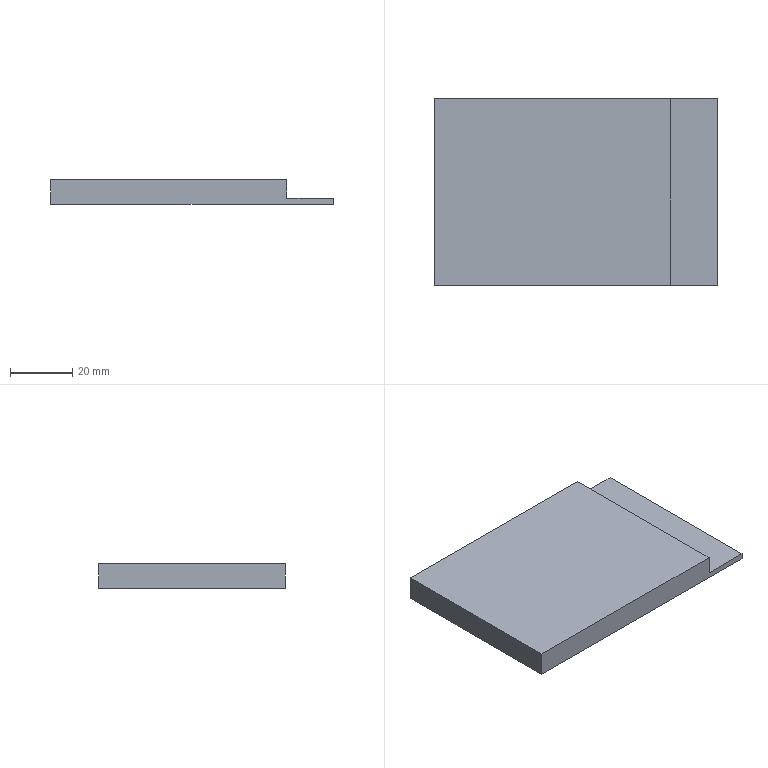Part | STEP file | Plate 4 | 1 solid | 8 faces | box 91 x 60 x 8 mm | volume 38280 mm3 | plane 8
STEP:
#1=CARTESIAN_POINT('',(45.5,30.,2.));
#2=VERTEX_POINT('',#1);
#3=CARTESIAN_POINT('',(45.5,30.,0.));
#4=VERTEX_POINT('',#3);
#5=CARTESIAN_POINT('',(45.5,30.,8.));
#6=DIRECTION('',(0.,0.,-1.));
#7=VECTOR('',#6,1000.);
#8=LINE('',#5,#7);
#9=EDGE_CURVE('',#2,#4,#8,.T.);
#10=ORIENTED_EDGE('',*,*,#9,.F.);
#11=CARTESIAN_POINT('',(45.5,-30.,2.));
#12=VERTEX_POINT('',#11);
#13=CARTESIAN_POINT('',(45.5,30.001,2.));
#14=DIRECTION('',(0.,-1.,0.));
#15=VECTOR('',#14,1000.);
#16=LINE('',#13,#15);
#17=EDGE_CURVE('',#2,#12,#16,.T.);
#18=ORIENTED_EDGE('',*,*,#17,.T.);
#19=CARTESIAN_POINT('',(45.5,-30.,0.));
#20=VERTEX_POINT('',#19);
#21=CARTESIAN_POINT('',(45.5,-30.,8.));
#22=DIRECTION('',(0.,0.,-1.));
#23=VECTOR('',#22,1000.);
#24=LINE('',#21,#23);
#25=EDGE_CURVE('',#12,#20,#24,.T.);
#26=ORIENTED_EDGE('',*,*,#25,.T.);
#27=CARTESIAN_POINT('',(45.5,-30.,0.));
#28=DIRECTION('',(0.,1.,0.));
#29=VECTOR('',#28,1000.);
#30=LINE('',#27,#29);
#31=EDGE_CURVE('',#20,#4,#30,.T.);
#32=ORIENTED_EDGE('',*,*,#31,.T.);
#33=EDGE_LOOP('',(#10,#18,#26,#32));
#34=FACE_OUTER_BOUND('',#33,.T.);
#35=CARTESIAN_POINT('',(45.5,-30.,8.));
#36=DIRECTION('',(-1.,0.,0.));
#37=DIRECTION('',(0.,0.,1.));
#38=AXIS2_PLACEMENT_3D('',#35,#36,#37);
#39=PLANE('',#38);
#40=ADVANCED_FACE('',(#34),#39,.F.);
#41=CARTESIAN_POINT('',(30.5,30.,2.));
#42=VERTEX_POINT('',#41);
#43=CARTESIAN_POINT('',(30.5,30.,8.));
#44=VERTEX_POINT('',#43);
#45=CARTESIAN_POINT('',(30.5,30.,8.));
#46=DIRECTION('',(0.,0.,1.));
#47=VECTOR('',#46,1000.);
#48=LINE('',#45,#47);
#49=EDGE_CURVE('',#42,#44,#48,.T.);
#50=ORIENTED_EDGE('',*,*,#49,.F.);
#51=CARTESIAN_POINT('',(45.5,30.,2.));
#52=DIRECTION('',(-1.,0.,0.));
#53=VECTOR('',#52,1000.);
#54=LINE('',#51,#53);
#55=EDGE_CURVE('',#2,#42,#54,.T.);
#56=ORIENTED_EDGE('',*,*,#55,.F.);
#57=ORIENTED_EDGE('',*,*,#9,.T.);
#58=CARTESIAN_POINT('',(-45.5,30.,0.));
#59=VERTEX_POINT('',#58);
#60=CARTESIAN_POINT('',(-45.5,30.,0.));
#61=DIRECTION('',(-1.,0.,0.));
#62=VECTOR('',#61,1000.);
#63=LINE('',#60,#62);
#64=EDGE_CURVE('',#4,#59,#63,.T.);
#65=ORIENTED_EDGE('',*,*,#64,.T.);
#66=CARTESIAN_POINT('',(-45.5,30.,8.));
#67=VERTEX_POINT('',#66);
#68=CARTESIAN_POINT('',(-45.5,30.,8.));
#69=DIRECTION('',(0.,0.,-1.));
#70=VECTOR('',#69,1000.);
#71=LINE('',#68,#70);
#72=EDGE_CURVE('',#67,#59,#71,.T.);
#73=ORIENTED_EDGE('',*,*,#72,.F.);
#74=CARTESIAN_POINT('',(-45.5,30.,8.));
#75=DIRECTION('',(-1.,0.,0.));
#76=VECTOR('',#75,1000.);
#77=LINE('',#74,#76);
#78=EDGE_CURVE('',#44,#67,#77,.T.);
#79=ORIENTED_EDGE('',*,*,#78,.F.);
#80=EDGE_LOOP('',(#50,#56,#57,#65,#73,#79));
#81=FACE_OUTER_BOUND('',#80,.T.);
#82=CARTESIAN_POINT('',(-45.5,30.,8.));
#83=DIRECTION('',(0.,-1.,0.));
#84=DIRECTION('',(0.,0.,-1.));
#85=AXIS2_PLACEMENT_3D('',#82,#83,#84);
#86=PLANE('',#85);
#87=ADVANCED_FACE('',(#81),#86,.F.);
#88=CARTESIAN_POINT('',(-45.5,-30.,0.));
#89=VERTEX_POINT('',#88);
#90=CARTESIAN_POINT('',(-45.5,-30.,0.));
#91=DIRECTION('',(0.,-1.,0.));
#92=VECTOR('',#91,1000.);
#93=LINE('',#90,#92);
#94=EDGE_CURVE('',#59,#89,#93,.T.);
#95=ORIENTED_EDGE('',*,*,#94,.T.);
#96=CARTESIAN_POINT('',(-45.5,-30.,8.));
#97=VERTEX_POINT('',#96);
#98=CARTESIAN_POINT('',(-45.5,-30.,8.));
#99=DIRECTION('',(0.,0.,-1.));
#100=VECTOR('',#99,1000.);
#101=LINE('',#98,#100);
#102=EDGE_CURVE('',#97,#89,#101,.T.);
#103=ORIENTED_EDGE('',*,*,#102,.F.);
#104=CARTESIAN_POINT('',(-45.5,-30.,8.));
#105=DIRECTION('',(0.,-1.,0.));
#106=VECTOR('',#105,1000.);
#107=LINE('',#104,#106);
#108=EDGE_CURVE('',#67,#97,#107,.T.);
#109=ORIENTED_EDGE('',*,*,#108,.F.);
#110=ORIENTED_EDGE('',*,*,#72,.T.);
#111=EDGE_LOOP('',(#95,#103,#109,#110));
#112=FACE_OUTER_BOUND('',#111,.T.);
#113=CARTESIAN_POINT('',(-45.5,-30.,8.));
#114=DIRECTION('',(1.,0.,0.));
#115=DIRECTION('',(0.,0.,-1.));
#116=AXIS2_PLACEMENT_3D('',#113,#114,#115);
#117=PLANE('',#116);
#118=ADVANCED_FACE('',(#112),#117,.F.);
#119=ORIENTED_EDGE('',*,*,#25,.F.);
#120=CARTESIAN_POINT('',(30.5,-30.,2.));
#121=VERTEX_POINT('',#120);
#122=CARTESIAN_POINT('',(45.5,-30.,2.));
#123=DIRECTION('',(1.,0.,0.));
#124=VECTOR('',#123,1000.);
#125=LINE('',#122,#124);
#126=EDGE_CURVE('',#121,#12,#125,.T.);
#127=ORIENTED_EDGE('',*,*,#126,.F.);
#128=CARTESIAN_POINT('',(30.5,-30.,8.));
#129=VERTEX_POINT('',#128);
#130=CARTESIAN_POINT('',(30.5,-30.,8.));
#131=DIRECTION('',(0.,0.,-1.));
#132=VECTOR('',#131,1000.);
#133=LINE('',#130,#132);
#134=EDGE_CURVE('',#129,#121,#133,.T.);
#135=ORIENTED_EDGE('',*,*,#134,.F.);
#136=CARTESIAN_POINT('',(-45.5,-30.,8.));
#137=DIRECTION('',(1.,0.,0.));
#138=VECTOR('',#137,1000.);
#139=LINE('',#136,#138);
#140=EDGE_CURVE('',#97,#129,#139,.T.);
#141=ORIENTED_EDGE('',*,*,#140,.F.);
#142=ORIENTED_EDGE('',*,*,#102,.T.);
#143=CARTESIAN_POINT('',(-45.5,-30.,0.));
#144=DIRECTION('',(1.,0.,0.));
#145=VECTOR('',#144,1000.);
#146=LINE('',#143,#145);
#147=EDGE_CURVE('',#89,#20,#146,.T.);
#148=ORIENTED_EDGE('',*,*,#147,.T.);
#149=EDGE_LOOP('',(#119,#127,#135,#141,#142,#148));
#150=FACE_OUTER_BOUND('',#149,.T.);
#151=CARTESIAN_POINT('',(-45.5,-30.,8.));
#152=DIRECTION('',(0.,1.,0.));
#153=DIRECTION('',(0.,0.,1.));
#154=AXIS2_PLACEMENT_3D('',#151,#152,#153);
#155=PLANE('',#154);
#156=ADVANCED_FACE('',(#150),#155,.F.);
#157=ORIENTED_EDGE('',*,*,#140,.T.);
#158=CARTESIAN_POINT('',(30.5,30.001,8.));
#159=DIRECTION('',(0.,-1.,0.));
#160=VECTOR('',#159,1000.);
#161=LINE('',#158,#160);
#162=EDGE_CURVE('',#44,#129,#161,.T.);
#163=ORIENTED_EDGE('',*,*,#162,.F.);
#164=ORIENTED_EDGE('',*,*,#78,.T.);
#165=ORIENTED_EDGE('',*,*,#108,.T.);
#166=EDGE_LOOP('',(#157,#163,#164,#165));
#167=FACE_OUTER_BOUND('',#166,.T.);
#168=CARTESIAN_POINT('',(0.,0.,8.));
#169=DIRECTION('',(0.,0.,-1.));
#170=DIRECTION('',(-1.,0.,0.));
#171=AXIS2_PLACEMENT_3D('',#168,#169,#170);
#172=PLANE('',#171);
#173=ADVANCED_FACE('',(#167),#172,.F.);
#174=ORIENTED_EDGE('',*,*,#31,.F.);
#175=ORIENTED_EDGE('',*,*,#147,.F.);
#176=ORIENTED_EDGE('',*,*,#94,.F.);
#177=ORIENTED_EDGE('',*,*,#64,.F.);
#178=EDGE_LOOP('',(#174,#175,#176,#177));
#179=FACE_OUTER_BOUND('',#178,.T.);
#180=CARTESIAN_POINT('',(0.,0.,0.));
#181=DIRECTION('',(0.,0.,-1.));
#182=DIRECTION('',(-1.,0.,0.));
#183=AXIS2_PLACEMENT_3D('',#180,#181,#182);
#184=PLANE('',#183);
#185=ADVANCED_FACE('',(#179),#184,.T.);
#186=ORIENTED_EDGE('',*,*,#55,.T.);
#187=CARTESIAN_POINT('',(30.5,30.001,2.));
#188=DIRECTION('',(0.,-1.,0.));
#189=VECTOR('',#188,1000.);
#190=LINE('',#187,#189);
#191=EDGE_CURVE('',#42,#121,#190,.T.);
#192=ORIENTED_EDGE('',*,*,#191,.T.);
#193=ORIENTED_EDGE('',*,*,#126,.T.);
#194=ORIENTED_EDGE('',*,*,#17,.F.);
#195=EDGE_LOOP('',(#186,#192,#193,#194));
#196=FACE_OUTER_BOUND('',#195,.T.);
#197=CARTESIAN_POINT('',(45.5,30.001,2.));
#198=DIRECTION('',(0.,0.,-1.));
#199=DIRECTION('',(-1.,0.,0.));
#200=AXIS2_PLACEMENT_3D('',#197,#198,#199);
#201=PLANE('',#200);
#202=ADVANCED_FACE('',(#196),#201,.F.);
#203=ORIENTED_EDGE('',*,*,#49,.T.);
#204=ORIENTED_EDGE('',*,*,#162,.T.);
#205=ORIENTED_EDGE('',*,*,#134,.T.);
#206=ORIENTED_EDGE('',*,*,#191,.F.);
#207=EDGE_LOOP('',(#203,#204,#205,#206));
#208=FACE_OUTER_BOUND('',#207,.T.);
#209=CARTESIAN_POINT('',(30.5,30.001,8.));
#210=DIRECTION('',(-1.,0.,0.));
#211=DIRECTION('',(0.,0.,1.));
#212=AXIS2_PLACEMENT_3D('',#209,#210,#211);
#213=PLANE('',#212);
#214=ADVANCED_FACE('',(#208),#213,.F.);
#215=CLOSED_SHELL('',(#40,#87,#118,#156,#173,#185,#202,#214));
#216=MANIFOLD_SOLID_BREP('',#215);
#217=CARTESIAN_POINT('',(0.,0.,0.));
#218=DIRECTION('',(0.,0.,1.));
#219=DIRECTION('',(1.,0.,0.));
#220=AXIS2_PLACEMENT_3D('',#217,#218,#219);
#221=(LENGTH_UNIT()NAMED_UNIT(*)SI_UNIT(.MILLI.,.METRE.));
#222=UNCERTAINTY_MEASURE_WITH_UNIT(LENGTH_MEASURE(0.00001),#221,'','');
#223=(NAMED_UNIT(*)PLANE_ANGLE_UNIT()SI_UNIT($,.RADIAN.));
#224=(NAMED_UNIT(*)SI_UNIT($,.STERADIAN.)SOLID_ANGLE_UNIT());
#225=(GEOMETRIC_REPRESENTATION_CONTEXT(3)GLOBAL_UNCERTAINTY_ASSIGNED_CONTEXT((#222))GLOBAL_UNIT_ASSIGNED_CONTEXT((#221,#223,#224))REPRESENTATION_CONTEXT('',''));
#226=ADVANCED_BREP_SHAPE_REPRESENTATION('',(#216,#220),#225);